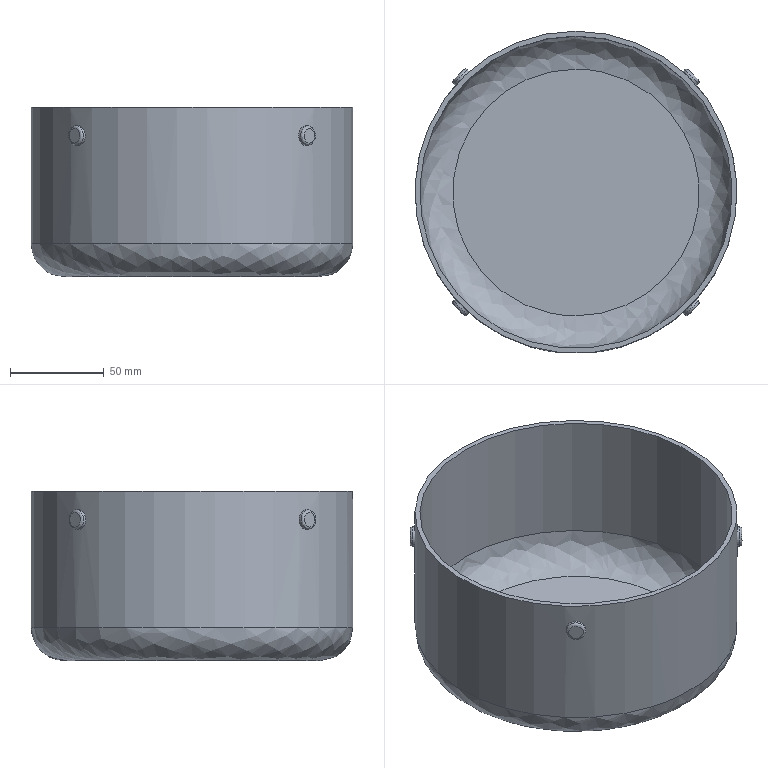Part | STEP file | Y2_FZ_80_1.step 3 | 1 solid | 19 faces | box 171.5 x 171.5 x 90 mm | volume 182303 mm3 | plane 7 | cylinder 6 | spline 6 | commonest cylinder face diameters 10.5 x4 166.25 x1 171.5 x1